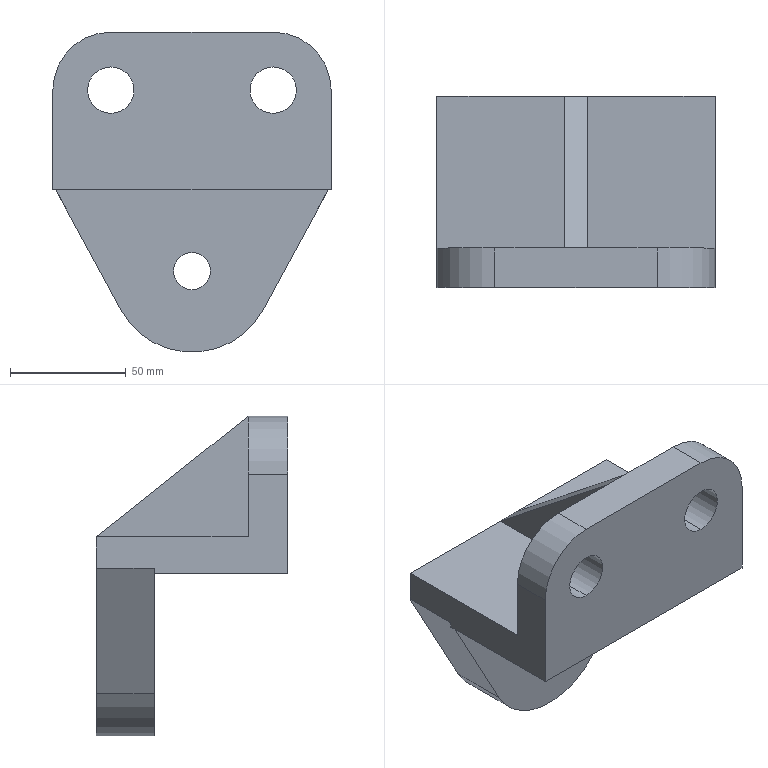Part | SolidWorks | features ICE 5, Extrusion 1 | 1 solid | 27 faces | box 120 x 82.471 x 138 mm | volume 396797 mm3 | plane 18 | cylinder 9 | commonest cylinder face diameters 20 x4 16 x2 50 x2 70 x1
STEP:
#1=CARTESIAN_POINT('',(-60.,57.471,-111.));
#2=VERTEX_POINT('',#1);
#3=CARTESIAN_POINT('',(-60.,57.471,-95.));
#4=VERTEX_POINT('',#3);
#5=CARTESIAN_POINT('',(-60.,57.471,-103.));
#6=DIRECTION('',(0.,1.,0.));
#7=DIRECTION('',(0.,0.,1.));
#8=AXIS2_PLACEMENT_3D('',#5,#6,#7);
#9=CIRCLE('',#8,8.);
#10=EDGE_CURVE('',#2,#4,#9,.T.);
#11=ORIENTED_EDGE('',*,*,#10,.F.);
#12=CARTESIAN_POINT('',(-60.,82.471,-111.));
#13=VERTEX_POINT('',#12);
#14=CARTESIAN_POINT('',(-60.,57.471,-111.));
#15=DIRECTION('',(0.,1.,0.));
#16=VECTOR('',#15,1000.);
#17=LINE('',#14,#16);
#18=EDGE_CURVE('',#2,#13,#17,.T.);
#19=ORIENTED_EDGE('',*,*,#18,.T.);
#20=CARTESIAN_POINT('',(-60.,82.471,-95.));
#21=VERTEX_POINT('',#20);
#22=CARTESIAN_POINT('',(-60.,82.471,-103.));
#23=DIRECTION('',(0.,1.,0.));
#24=DIRECTION('',(0.,0.,1.));
#25=AXIS2_PLACEMENT_3D('',#22,#23,#24);
#26=CIRCLE('',#25,8.);
#27=EDGE_CURVE('',#13,#21,#26,.T.);
#28=ORIENTED_EDGE('',*,*,#27,.T.);
#29=CARTESIAN_POINT('',(-60.,57.471,-95.));
#30=DIRECTION('',(0.,1.,0.));
#31=VECTOR('',#30,1000.);
#32=LINE('',#29,#31);
#33=EDGE_CURVE('',#4,#21,#32,.T.);
#34=ORIENTED_EDGE('',*,*,#33,.F.);
#35=EDGE_LOOP('',(#11,#19,#28,#34));
#36=FACE_OUTER_BOUND('',#35,.T.);
#37=CARTESIAN_POINT('',(-60.,57.471,-103.));
#38=DIRECTION('',(0.,1.,0.));
#39=DIRECTION('',(0.,0.,1.));
#40=AXIS2_PLACEMENT_3D('',#37,#38,#39);
#41=CYLINDRICAL_SURFACE('',#40,8.);
#42=ADVANCED_FACE('',(#36),#41,.F.);
#43=CARTESIAN_POINT('',(-25.,17.,-15.));
#44=VERTEX_POINT('',#43);
#45=CARTESIAN_POINT('',(-25.,17.,-35.));
#46=VERTEX_POINT('',#45);
#47=CARTESIAN_POINT('',(-25.,17.,-25.));
#48=DIRECTION('',(0.,-1.,0.));
#49=DIRECTION('',(0.,0.,-1.));
#50=AXIS2_PLACEMENT_3D('',#47,#48,#49);
#51=CIRCLE('',#50,10.);
#52=EDGE_CURVE('',#44,#46,#51,.T.);
#53=ORIENTED_EDGE('',*,*,#52,.F.);
#54=CARTESIAN_POINT('',(-25.,0.,-15.));
#55=VERTEX_POINT('',#54);
#56=CARTESIAN_POINT('',(-25.,55.,-15.));
#57=DIRECTION('',(0.,-1.,0.));
#58=VECTOR('',#57,1000.);
#59=LINE('',#56,#58);
#60=EDGE_CURVE('',#44,#55,#59,.T.);
#61=ORIENTED_EDGE('',*,*,#60,.T.);
#62=CARTESIAN_POINT('',(-25.,0.,-35.));
#63=VERTEX_POINT('',#62);
#64=CARTESIAN_POINT('',(-25.,0.,-25.));
#65=DIRECTION('',(0.,-1.,0.));
#66=DIRECTION('',(0.,0.,-1.));
#67=AXIS2_PLACEMENT_3D('',#64,#65,#66);
#68=CIRCLE('',#67,10.);
#69=EDGE_CURVE('',#55,#63,#68,.T.);
#70=ORIENTED_EDGE('',*,*,#69,.T.);
#71=CARTESIAN_POINT('',(-25.,55.,-35.));
#72=DIRECTION('',(0.,-1.,0.));
#73=VECTOR('',#72,1000.);
#74=LINE('',#71,#73);
#75=EDGE_CURVE('',#46,#63,#74,.T.);
#76=ORIENTED_EDGE('',*,*,#75,.F.);
#77=EDGE_LOOP('',(#53,#61,#70,#76));
#78=FACE_OUTER_BOUND('',#77,.T.);
#79=CARTESIAN_POINT('',(-25.,55.,-25.));
#80=DIRECTION('',(0.,-1.,0.));
#81=DIRECTION('',(0.,0.,-1.));
#82=AXIS2_PLACEMENT_3D('',#79,#80,#81);
#83=CYLINDRICAL_SURFACE('',#82,10.);
#84=ADVANCED_FACE('',(#78),#83,.F.);
#85=CARTESIAN_POINT('',(-95.,17.,-15.));
#86=VERTEX_POINT('',#85);
#87=CARTESIAN_POINT('',(-95.,17.,-35.));
#88=VERTEX_POINT('',#87);
#89=CARTESIAN_POINT('',(-95.,17.,-25.));
#90=DIRECTION('',(0.,-1.,0.));
#91=DIRECTION('',(0.,0.,-1.));
#92=AXIS2_PLACEMENT_3D('',#89,#90,#91);
#93=CIRCLE('',#92,10.);
#94=EDGE_CURVE('',#86,#88,#93,.T.);
#95=ORIENTED_EDGE('',*,*,#94,.F.);
#96=CARTESIAN_POINT('',(-95.,0.,-15.));
#97=VERTEX_POINT('',#96);
#98=CARTESIAN_POINT('',(-95.,55.,-15.));
#99=DIRECTION('',(0.,-1.,0.));
#100=VECTOR('',#99,1000.);
#101=LINE('',#98,#100);
#102=EDGE_CURVE('',#86,#97,#101,.T.);
#103=ORIENTED_EDGE('',*,*,#102,.T.);
#104=CARTESIAN_POINT('',(-95.,0.,-35.));
#105=VERTEX_POINT('',#104);
#106=CARTESIAN_POINT('',(-95.,0.,-25.));
#107=DIRECTION('',(0.,-1.,0.));
#108=DIRECTION('',(0.,0.,-1.));
#109=AXIS2_PLACEMENT_3D('',#106,#107,#108);
#110=CIRCLE('',#109,10.);
#111=EDGE_CURVE('',#97,#105,#110,.T.);
#112=ORIENTED_EDGE('',*,*,#111,.T.);
#113=CARTESIAN_POINT('',(-95.,55.,-35.));
#114=DIRECTION('',(0.,-1.,0.));
#115=VECTOR('',#114,1000.);
#116=LINE('',#113,#115);
#117=EDGE_CURVE('',#88,#105,#116,.T.);
#118=ORIENTED_EDGE('',*,*,#117,.F.);
#119=EDGE_LOOP('',(#95,#103,#112,#118));
#120=FACE_OUTER_BOUND('',#119,.T.);
#121=CARTESIAN_POINT('',(-95.,55.,-25.));
#122=DIRECTION('',(0.,-1.,0.));
#123=DIRECTION('',(0.,0.,-1.));
#124=AXIS2_PLACEMENT_3D('',#121,#122,#123);
#125=CYLINDRICAL_SURFACE('',#124,10.);
#126=ADVANCED_FACE('',(#120),#125,.F.);
#127=CARTESIAN_POINT('',(-60.,82.471,-103.));
#128=DIRECTION('',(0.,1.,0.));
#129=DIRECTION('',(0.,0.,1.));
#130=AXIS2_PLACEMENT_3D('',#127,#128,#129);
#131=CIRCLE('',#130,8.);
#132=EDGE_CURVE('',#21,#13,#131,.T.);
#133=ORIENTED_EDGE('',*,*,#132,.F.);
#134=ORIENTED_EDGE('',*,*,#27,.F.);
#135=EDGE_LOOP('',(#133,#134));
#136=FACE_BOUND('',#135,.T.);
#137=CARTESIAN_POINT('',(-29.216,82.471,-119.654));
#138=VERTEX_POINT('',#137);
#139=CARTESIAN_POINT('',(-90.784,82.471,-119.654));
#140=VERTEX_POINT('',#139);
#141=CARTESIAN_POINT('',(-60.,82.471,-103.));
#142=DIRECTION('',(0.,1.,0.));
#143=DIRECTION('',(0.,0.,1.));
#144=AXIS2_PLACEMENT_3D('',#141,#142,#143);
#145=CIRCLE('',#144,35.);
#146=EDGE_CURVE('',#138,#140,#145,.T.);
#147=ORIENTED_EDGE('',*,*,#146,.T.);
#148=CARTESIAN_POINT('',(-120.,82.471,-65.649));
#149=VERTEX_POINT('',#148);
#150=CARTESIAN_POINT('',(-120.306,82.471,-65.085));
#151=DIRECTION('',(0.4758,0.,-0.8795));
#152=VECTOR('',#151,1000.);
#153=LINE('',#150,#152);
#154=EDGE_CURVE('',#149,#140,#153,.T.);
#155=ORIENTED_EDGE('',*,*,#154,.F.);
#156=CARTESIAN_POINT('',(-120.,82.471,-52.));
#157=VERTEX_POINT('',#156);
#158=CARTESIAN_POINT('',(-120.,82.471,0.));
#159=DIRECTION('',(0.,0.,1.));
#160=VECTOR('',#159,1000.);
#161=LINE('',#158,#160);
#162=EDGE_CURVE('',#149,#157,#161,.T.);
#163=ORIENTED_EDGE('',*,*,#162,.T.);
#164=CARTESIAN_POINT('',(-65.,82.471,-52.));
#165=VERTEX_POINT('',#164);
#166=CARTESIAN_POINT('',(-120.,82.471,-52.));
#167=DIRECTION('',(1.,0.,0.));
#168=VECTOR('',#167,1000.);
#169=LINE('',#166,#168);
#170=EDGE_CURVE('',#157,#165,#169,.T.);
#171=ORIENTED_EDGE('',*,*,#170,.T.);
#172=CARTESIAN_POINT('',(-55.,82.471,-52.));
#173=VERTEX_POINT('',#172);
#174=CARTESIAN_POINT('',(-120.,82.471,-52.));
#175=DIRECTION('',(1.,0.,0.));
#176=VECTOR('',#175,1000.);
#177=LINE('',#174,#176);
#178=EDGE_CURVE('',#165,#173,#177,.T.);
#179=ORIENTED_EDGE('',*,*,#178,.T.);
#180=CARTESIAN_POINT('',(0.,82.471,-52.));
#181=VERTEX_POINT('',#180);
#182=CARTESIAN_POINT('',(-55.,82.471,-52.));
#183=DIRECTION('',(1.,0.,0.));
#184=VECTOR('',#183,1000.);
#185=LINE('',#182,#184);
#186=EDGE_CURVE('',#173,#181,#185,.T.);
#187=ORIENTED_EDGE('',*,*,#186,.T.);
#188=CARTESIAN_POINT('',(0.,82.471,-65.649));
#189=VERTEX_POINT('',#188);
#190=CARTESIAN_POINT('',(0.,82.471,0.));
#191=DIRECTION('',(0.,0.,1.));
#192=VECTOR('',#191,1000.);
#193=LINE('',#190,#192);
#194=EDGE_CURVE('',#189,#181,#193,.T.);
#195=ORIENTED_EDGE('',*,*,#194,.F.);
#196=CARTESIAN_POINT('',(27.475,82.471,-14.864));
#197=DIRECTION('',(-0.4758,0.,-0.8795));
#198=VECTOR('',#197,1000.);
#199=LINE('',#196,#198);
#200=EDGE_CURVE('',#189,#138,#199,.T.);
#201=ORIENTED_EDGE('',*,*,#200,.T.);
#202=EDGE_LOOP('',(#147,#155,#163,#171,#179,#187,#195,#201));
#203=FACE_OUTER_BOUND('',#202,.T.);
#204=CARTESIAN_POINT('',(-120.,82.471,0.));
#205=DIRECTION('',(0.,1.,0.));
#206=DIRECTION('',(0.,0.,1.));
#207=AXIS2_PLACEMENT_3D('',#204,#205,#206);
#208=PLANE('',#207);
#209=ADVANCED_FACE('',(#136,#203),#208,.T.);
#210=CARTESIAN_POINT('',(-60.,57.471,-103.));
#211=DIRECTION('',(0.,1.,0.));
#212=DIRECTION('',(0.,0.,1.));
#213=AXIS2_PLACEMENT_3D('',#210,#211,#212);
#214=CIRCLE('',#213,8.);
#215=EDGE_CURVE('',#4,#2,#214,.T.);
#216=ORIENTED_EDGE('',*,*,#215,.T.);
#217=ORIENTED_EDGE('',*,*,#10,.T.);
#218=EDGE_LOOP('',(#216,#217));
#219=FACE_BOUND('',#218,.T.);
#220=CARTESIAN_POINT('',(-118.728,57.471,-68.));
#221=VERTEX_POINT('',#220);
#222=CARTESIAN_POINT('',(-90.784,57.471,-119.654));
#223=VERTEX_POINT('',#222);
#224=CARTESIAN_POINT('',(-120.306,57.471,-65.085));
#225=DIRECTION('',(0.4758,0.,-0.8795));
#226=VECTOR('',#225,1000.);
#227=LINE('',#224,#226);
#228=EDGE_CURVE('',#221,#223,#227,.T.);
#229=ORIENTED_EDGE('',*,*,#228,.T.);
#230=CARTESIAN_POINT('',(-29.216,57.471,-119.654));
#231=VERTEX_POINT('',#230);
#232=CARTESIAN_POINT('',(-60.,57.471,-103.));
#233=DIRECTION('',(0.,1.,0.));
#234=DIRECTION('',(0.,0.,1.));
#235=AXIS2_PLACEMENT_3D('',#232,#233,#234);
#236=CIRCLE('',#235,35.);
#237=EDGE_CURVE('',#231,#223,#236,.T.);
#238=ORIENTED_EDGE('',*,*,#237,.F.);
#239=CARTESIAN_POINT('',(-1.272,57.471,-68.));
#240=VERTEX_POINT('',#239);
#241=CARTESIAN_POINT('',(-57.448,57.471,-171.84));
#242=DIRECTION('',(0.4758,0.,0.8795));
#243=VECTOR('',#242,1000.);
#244=LINE('',#241,#243);
#245=EDGE_CURVE('',#231,#240,#244,.T.);
#246=ORIENTED_EDGE('',*,*,#245,.T.);
#247=CARTESIAN_POINT('',(-120.,57.471,-68.));
#248=DIRECTION('',(1.,0.,0.));
#249=VECTOR('',#248,1000.);
#250=LINE('',#247,#249);
#251=EDGE_CURVE('',#221,#240,#250,.T.);
#252=ORIENTED_EDGE('',*,*,#251,.F.);
#253=EDGE_LOOP('',(#229,#238,#246,#252));
#254=FACE_OUTER_BOUND('',#253,.T.);
#255=CARTESIAN_POINT('',(-120.,57.471,-138.));
#256=DIRECTION('',(0.,-1.,0.));
#257=DIRECTION('',(0.,0.,-1.));
#258=AXIS2_PLACEMENT_3D('',#255,#256,#257);
#259=PLANE('',#258);
#260=ADVANCED_FACE('',(#219,#254),#259,.T.);
#261=CARTESIAN_POINT('',(0.,57.471,-65.649));
#262=VERTEX_POINT('',#261);
#263=CARTESIAN_POINT('',(0.,57.471,-68.));
#264=VERTEX_POINT('',#263);
#265=CARTESIAN_POINT('',(0.,57.471,0.));
#266=DIRECTION('',(0.,0.,-1.));
#267=VECTOR('',#266,1000.);
#268=LINE('',#265,#267);
#269=EDGE_CURVE('',#262,#264,#268,.T.);
#270=ORIENTED_EDGE('',*,*,#269,.F.);
#271=CARTESIAN_POINT('',(0.,57.471,-65.649));
#272=DIRECTION('',(0.,1.,0.));
#273=VECTOR('',#272,1000.);
#274=LINE('',#271,#273);
#275=EDGE_CURVE('',#262,#189,#274,.T.);
#276=ORIENTED_EDGE('',*,*,#275,.T.);
#277=ORIENTED_EDGE('',*,*,#194,.T.);
#278=CARTESIAN_POINT('',(0.,17.,-52.));
#279=VERTEX_POINT('',#278);
#280=CARTESIAN_POINT('',(0.,17.,-52.));
#281=DIRECTION('',(0.,1.,0.));
#282=VECTOR('',#281,1000.);
#283=LINE('',#280,#282);
#284=EDGE_CURVE('',#279,#181,#283,.T.);
#285=ORIENTED_EDGE('',*,*,#284,.F.);
#286=CARTESIAN_POINT('',(0.,17.,-25.));
#287=VERTEX_POINT('',#286);
#288=CARTESIAN_POINT('',(0.,17.,0.));
#289=DIRECTION('',(0.,0.,-1.));
#290=VECTOR('',#289,1000.);
#291=LINE('',#288,#290);
#292=EDGE_CURVE('',#287,#279,#291,.T.);
#293=ORIENTED_EDGE('',*,*,#292,.F.);
#294=CARTESIAN_POINT('',(0.,0.,-25.));
#295=VERTEX_POINT('',#294);
#296=CARTESIAN_POINT('',(0.,55.,-25.));
#297=DIRECTION('',(0.,-1.,0.));
#298=VECTOR('',#297,1000.);
#299=LINE('',#296,#298);
#300=EDGE_CURVE('',#287,#295,#299,.T.);
#301=ORIENTED_EDGE('',*,*,#300,.T.);
#302=CARTESIAN_POINT('',(0.,0.,-68.));
#303=VERTEX_POINT('',#302);
#304=CARTESIAN_POINT('',(0.,0.,0.));
#305=DIRECTION('',(0.,0.,-1.));
#306=VECTOR('',#305,1000.);
#307=LINE('',#304,#306);
#308=EDGE_CURVE('',#295,#303,#307,.T.);
#309=ORIENTED_EDGE('',*,*,#308,.T.);
#310=CARTESIAN_POINT('',(0.,0.,-68.));
#311=DIRECTION('',(0.,1.,0.));
#312=VECTOR('',#311,1000.);
#313=LINE('',#310,#312);
#314=EDGE_CURVE('',#303,#264,#313,.T.);
#315=ORIENTED_EDGE('',*,*,#314,.T.);
#316=EDGE_LOOP('',(#270,#276,#277,#285,#293,#301,#309,#315));
#317=FACE_OUTER_BOUND('',#316,.T.);
#318=CARTESIAN_POINT('',(0.,0.,0.));
#319=DIRECTION('',(1.,0.,0.));
#320=DIRECTION('',(0.,0.,-1.));
#321=AXIS2_PLACEMENT_3D('',#318,#319,#320);
#322=PLANE('',#321);
#323=ADVANCED_FACE('',(#317),#322,.T.);
#324=CARTESIAN_POINT('',(-120.,0.,-68.));
#325=VERTEX_POINT('',#324);
#326=CARTESIAN_POINT('',(-120.,57.471,-68.));
#327=VERTEX_POINT('',#326);
#328=CARTESIAN_POINT('',(-120.,0.,-68.));
#329=DIRECTION('',(0.,1.,0.));
#330=VECTOR('',#329,1000.);
#331=LINE('',#328,#330);
#332=EDGE_CURVE('',#325,#327,#331,.T.);
#333=ORIENTED_EDGE('',*,*,#332,.T.);
#334=CARTESIAN_POINT('',(-120.,57.471,-68.));
#335=DIRECTION('',(1.,0.,0.));
#336=VECTOR('',#335,1000.);
#337=LINE('',#334,#336);
#338=EDGE_CURVE('',#327,#221,#337,.T.);
#339=ORIENTED_EDGE('',*,*,#338,.T.);
#340=ORIENTED_EDGE('',*,*,#251,.T.);
#341=CARTESIAN_POINT('',(-120.,57.471,-68.));
#342=DIRECTION('',(1.,0.,0.));
#343=VECTOR('',#342,1000.);
#344=LINE('',#341,#343);
#345=EDGE_CURVE('',#240,#264,#344,.T.);
#346=ORIENTED_EDGE('',*,*,#345,.T.);
#347=ORIENTED_EDGE('',*,*,#314,.F.);
#348=CARTESIAN_POINT('',(-120.,0.,-68.));
#349=DIRECTION('',(1.,0.,0.));
#350=VECTOR('',#349,1000.);
#351=LINE('',#348,#350);
#352=EDGE_CURVE('',#325,#303,#351,.T.);
#353=ORIENTED_EDGE('',*,*,#352,.F.);
#354=EDGE_LOOP('',(#333,#339,#340,#346,#347,#353));
#355=FACE_OUTER_BOUND('',#354,.T.);
#356=CARTESIAN_POINT('',(-120.,0.,-68.));
#357=DIRECTION('',(0.,0.,-1.));
#358=DIRECTION('',(-1.,0.,0.));
#359=AXIS2_PLACEMENT_3D('',#356,#357,#358);
#360=PLANE('',#359);
#361=ADVANCED_FACE('',(#355),#360,.T.);
#362=CARTESIAN_POINT('',(-25.,0.,-25.));
#363=DIRECTION('',(0.,-1.,0.));
#364=DIRECTION('',(0.,0.,-1.));
#365=AXIS2_PLACEMENT_3D('',#362,#363,#364);
#366=CIRCLE('',#365,10.);
#367=EDGE_CURVE('',#63,#55,#366,.T.);
#368=ORIENTED_EDGE('',*,*,#367,.F.);
#369=ORIENTED_EDGE('',*,*,#69,.F.);
#370=EDGE_LOOP('',(#368,#369));
#371=FACE_BOUND('',#370,.T.);
#372=CARTESIAN_POINT('',(-95.,0.,-25.));
#373=DIRECTION('',(0.,-1.,0.));
#374=DIRECTION('',(0.,0.,-1.));
#375=AXIS2_PLACEMENT_3D('',#372,#373,#374);
#376=CIRCLE('',#375,10.);
#377=EDGE_CURVE('',#105,#97,#376,.T.);
#378=ORIENTED_EDGE('',*,*,#377,.F.);
#379=ORIENTED_EDGE('',*,*,#111,.F.);
#380=EDGE_LOOP('',(#378,#379));
#381=FACE_BOUND('',#380,.T.);
#382=ORIENTED_EDGE('',*,*,#308,.F.);
#383=CARTESIAN_POINT('',(-25.,0.,0.));
#384=VERTEX_POINT('',#383);
#385=CARTESIAN_POINT('',(-25.,0.,-25.));
#386=DIRECTION('',(0.,-1.,0.));
#387=DIRECTION('',(0.,0.,-1.));
#388=AXIS2_PLACEMENT_3D('',#385,#386,#387);
#389=CIRCLE('',#388,25.);
#390=EDGE_CURVE('',#295,#384,#389,.T.);
#391=ORIENTED_EDGE('',*,*,#390,.T.);
#392=CARTESIAN_POINT('',(-95.,0.,0.));
#393=VERTEX_POINT('',#392);
#394=CARTESIAN_POINT('',(-120.,0.,0.));
#395=DIRECTION('',(1.,0.,0.));
#396=VECTOR('',#395,1000.);
#397=LINE('',#394,#396);
#398=EDGE_CURVE('',#393,#384,#397,.T.);
#399=ORIENTED_EDGE('',*,*,#398,.F.);
#400=CARTESIAN_POINT('',(-120.,0.,-25.));
#401=VERTEX_POINT('',#400);
#402=CARTESIAN_POINT('',(-95.,0.,-25.));
#403=DIRECTION('',(0.,-1.,0.));
#404=DIRECTION('',(0.,0.,-1.));
#405=AXIS2_PLACEMENT_3D('',#402,#403,#404);
#406=CIRCLE('',#405,25.);
#407=EDGE_CURVE('',#393,#401,#406,.T.);
#408=ORIENTED_EDGE('',*,*,#407,.T.);
#409=CARTESIAN_POINT('',(-120.,0.,0.));
#410=DIRECTION('',(0.,0.,-1.));
#411=VECTOR('',#410,1000.);
#412=LINE('',#409,#411);
#413=EDGE_CURVE('',#401,#325,#412,.T.);
#414=ORIENTED_EDGE('',*,*,#413,.T.);
#415=ORIENTED_EDGE('',*,*,#352,.T.);
#416=EDGE_LOOP('',(#382,#391,#399,#408,#414,#415));
#417=FACE_OUTER_BOUND('',#416,.T.);
#418=CARTESIAN_POINT('',(-120.,0.,0.));
#419=DIRECTION('',(0.,-1.,0.));
#420=DIRECTION('',(0.,0.,-1.));
#421=AXIS2_PLACEMENT_3D('',#418,#419,#420);
#422=PLANE('',#421);
#423=ADVANCED_FACE('',(#371,#381,#417),#422,.T.);
#424=CARTESIAN_POINT('',(-25.,17.,-25.));
#425=DIRECTION('',(0.,-1.,0.));
#426=DIRECTION('',(0.,0.,-1.));
#427=AXIS2_PLACEMENT_3D('',#424,#425,#426);
#428=CIRCLE('',#427,10.);
#429=EDGE_CURVE('',#46,#44,#428,.T.);
#430=ORIENTED_EDGE('',*,*,#429,.T.);
#431=ORIENTED_EDGE('',*,*,#52,.T.);
#432=EDGE_LOOP('',(#430,#431));
#433=FACE_BOUND('',#432,.T.);
#434=CARTESIAN_POINT('',(-25.,17.,0.));
#435=VERTEX_POINT('',#434);
#436=CARTESIAN_POINT('',(-25.,17.,-25.));
#437=DIRECTION('',(0.,-1.,0.));
#438=DIRECTION('',(0.,0.,-1.));
#439=AXIS2_PLACEMENT_3D('',#436,#437,#438);
#440=CIRCLE('',#439,25.);
#441=EDGE_CURVE('',#287,#435,#440,.T.);
#442=ORIENTED_EDGE('',*,*,#441,.F.);
#443=ORIENTED_EDGE('',*,*,#292,.T.);
#444=CARTESIAN_POINT('',(-55.,17.,-52.));
#445=VERTEX_POINT('',#444);
#446=CARTESIAN_POINT('',(-55.,17.,-52.));
#447=DIRECTION('',(1.,0.,0.));
#448=VECTOR('',#447,1000.);
#449=LINE('',#446,#448);
#450=EDGE_CURVE('',#445,#279,#449,.T.);
#451=ORIENTED_EDGE('',*,*,#450,.F.);
#452=CARTESIAN_POINT('',(-55.,17.,0.));
#453=VERTEX_POINT('',#452);
#454=CARTESIAN_POINT('',(-55.,17.,0.));
#455=DIRECTION('',(0.,0.,-1.));
#456=VECTOR('',#455,1000.);
#457=LINE('',#454,#456);
#458=EDGE_CURVE('',#453,#445,#457,.T.);
#459=ORIENTED_EDGE('',*,*,#458,.F.);
#460=CARTESIAN_POINT('',(-55.,17.,0.));
#461=DIRECTION('',(1.,0.,0.));
#462=VECTOR('',#461,1000.);
#463=LINE('',#460,#462);
#464=EDGE_CURVE('',#453,#435,#463,.T.);
#465=ORIENTED_EDGE('',*,*,#464,.T.);
#466=EDGE_LOOP('',(#442,#443,#451,#459,#465));
#467=FACE_OUTER_BOUND('',#466,.T.);
#468=CARTESIAN_POINT('',(-55.,17.,0.));
#469=DIRECTION('',(0.,-1.,0.));
#470=DIRECTION('',(0.,0.,-1.));
#471=AXIS2_PLACEMENT_3D('',#468,#469,#470);
#472=PLANE('',#471);
#473=ADVANCED_FACE('',(#433,#467),#472,.F.);
#474=CARTESIAN_POINT('',(-25.,55.,0.));
#475=DIRECTION('',(0.,-1.,0.));
#476=VECTOR('',#475,1000.);
#477=LINE('',#474,#476);
#478=EDGE_CURVE('',#435,#384,#477,.T.);
#479=ORIENTED_EDGE('',*,*,#478,.F.);
#480=ORIENTED_EDGE('',*,*,#464,.F.);
#481=CARTESIAN_POINT('',(-65.,17.,0.));
#482=VERTEX_POINT('',#481);
#483=CARTESIAN_POINT('',(-120.,17.,0.));
#484=DIRECTION('',(1.,0.,0.));
#485=VECTOR('',#484,1000.);
#486=LINE('',#483,#485);
#487=EDGE_CURVE('',#482,#453,#486,.T.);
#488=ORIENTED_EDGE('',*,*,#487,.F.);
#489=CARTESIAN_POINT('',(-95.,17.,0.));
#490=VERTEX_POINT('',#489);
#491=CARTESIAN_POINT('',(-120.,17.,0.));
#492=DIRECTION('',(1.,0.,0.));
#493=VECTOR('',#492,1000.);
#494=LINE('',#491,#493);
#495=EDGE_CURVE('',#490,#482,#494,.T.);
#496=ORIENTED_EDGE('',*,*,#495,.F.);
#497=CARTESIAN_POINT('',(-95.,55.,0.));
#498=DIRECTION('',(0.,-1.,0.));
#499=VECTOR('',#498,1000.);
#500=LINE('',#497,#499);
#501=EDGE_CURVE('',#490,#393,#500,.T.);
#502=ORIENTED_EDGE('',*,*,#501,.T.);
#503=ORIENTED_EDGE('',*,*,#398,.T.);
#504=EDGE_LOOP('',(#479,#480,#488,#496,#502,#503));
#505=FACE_OUTER_BOUND('',#504,.T.);
#506=CARTESIAN_POINT('',(-120.,0.,0.));
#507=DIRECTION('',(0.,0.,1.));
#508=DIRECTION('',(0.,-1.,0.));
#509=AXIS2_PLACEMENT_3D('',#506,#507,#508);
#510=PLANE('',#509);
#511=ADVANCED_FACE('',(#505),#510,.T.);
#512=ORIENTED_EDGE('',*,*,#162,.F.);
#513=CARTESIAN_POINT('',(-120.,57.471,-65.649));
#514=VERTEX_POINT('',#513);
#515=CARTESIAN_POINT('',(-120.,57.471,-65.649));
#516=DIRECTION('',(0.,1.,0.));
#517=VECTOR('',#516,1000.);
#518=LINE('',#515,#517);
#519=EDGE_CURVE('',#514,#149,#518,.T.);
#520=ORIENTED_EDGE('',*,*,#519,.F.);
#521=CARTESIAN_POINT('',(-120.,57.471,0.));
#522=DIRECTION('',(0.,0.,1.));
#523=VECTOR('',#522,1000.);
#524=LINE('',#521,#523);
#525=EDGE_CURVE('',#327,#514,#524,.T.);
#526=ORIENTED_EDGE('',*,*,#525,.F.);
#527=ORIENTED_EDGE('',*,*,#332,.F.);
#528=ORIENTED_EDGE('',*,*,#413,.F.);
#529=CARTESIAN_POINT('',(-120.,17.,-25.));
#530=VERTEX_POINT('',#529);
#531=CARTESIAN_POINT('',(-120.,55.,-25.));
#532=DIRECTION('',(0.,-1.,0.));
#533=VECTOR('',#532,1000.);
#534=LINE('',#531,#533);
#535=EDGE_CURVE('',#530,#401,#534,.T.);
#536=ORIENTED_EDGE('',*,*,#535,.F.);
#537=CARTESIAN_POINT('',(-120.,17.,-52.));
#538=VERTEX_POINT('',#537);
#539=CARTESIAN_POINT('',(-120.,17.,0.));
#540=DIRECTION('',(0.,0.,1.));
#541=VECTOR('',#540,1000.);
#542=LINE('',#539,#541);
#543=EDGE_CURVE('',#538,#530,#542,.T.);
#544=ORIENTED_EDGE('',*,*,#543,.F.);
#545=CARTESIAN_POINT('',(-120.,17.,-52.));
#546=DIRECTION('',(0.,-1.,0.));
#547=VECTOR('',#546,1000.);
#548=LINE('',#545,#547);
#549=EDGE_CURVE('',#157,#538,#548,.T.);
#550=ORIENTED_EDGE('',*,*,#549,.F.);
#551=EDGE_LOOP('',(#512,#520,#526,#527,#528,#536,#544,#550));
#552=FACE_OUTER_BOUND('',#551,.T.);
#553=CARTESIAN_POINT('',(-120.,0.,0.));
#554=DIRECTION('',(1.,0.,0.));
#555=DIRECTION('',(0.,0.,-1.));
#556=AXIS2_PLACEMENT_3D('',#553,#554,#555);
#557=PLANE('',#556);
#558=ADVANCED_FACE('',(#552),#557,.F.);
#559=CARTESIAN_POINT('',(-95.,17.,-25.));
#560=DIRECTION('',(0.,-1.,0.));
#561=DIRECTION('',(0.,0.,-1.));
#562=AXIS2_PLACEMENT_3D('',#559,#560,#561);
#563=CIRCLE('',#562,10.);
#564=EDGE_CURVE('',#88,#86,#563,.T.);
#565=ORIENTED_EDGE('',*,*,#564,.T.);
#566=ORIENTED_EDGE('',*,*,#94,.T.);
#567=EDGE_LOOP('',(#565,#566));
#568=FACE_BOUND('',#567,.T.);
#569=CARTESIAN_POINT('',(-95.,17.,-25.));
#570=DIRECTION('',(0.,-1.,0.));
#571=DIRECTION('',(0.,0.,-1.));
#572=AXIS2_PLACEMENT_3D('',#569,#570,#571);
#573=CIRCLE('',#572,25.);
#574=EDGE_CURVE('',#490,#530,#573,.T.);
#575=ORIENTED_EDGE('',*,*,#574,.F.);
#576=ORIENTED_EDGE('',*,*,#495,.T.);
#577=CARTESIAN_POINT('',(-65.,17.,-52.));
#578=VERTEX_POINT('',#577);
#579=CARTESIAN_POINT('',(-65.,17.,0.));
#580=DIRECTION('',(0.,0.,1.));
#581=VECTOR('',#580,1000.);
#582=LINE('',#579,#581);
#583=EDGE_CURVE('',#578,#482,#582,.T.);
#584=ORIENTED_EDGE('',*,*,#583,.F.);
#585=CARTESIAN_POINT('',(-65.,17.,-52.));
#586=DIRECTION('',(-1.,0.,0.));
#587=VECTOR('',#586,1000.);
#588=LINE('',#585,#587);
#589=EDGE_CURVE('',#578,#538,#588,.T.);
#590=ORIENTED_EDGE('',*,*,#589,.T.);
#591=ORIENTED_EDGE('',*,*,#543,.T.);
#592=EDGE_LOOP('',(#575,#576,#584,#590,#591));
#593=FACE_OUTER_BOUND('',#592,.T.);
#594=CARTESIAN_POINT('',(-65.,17.,0.));
#595=DIRECTION('',(0.,-1.,0.));
#596=DIRECTION('',(0.,0.,-1.));
#597=AXIS2_PLACEMENT_3D('',#594,#595,#596);
#598=PLANE('',#597);
#599=ADVANCED_FACE('',(#568,#593),#598,.F.);
#600=ORIENTED_EDGE('',*,*,#178,.F.);
#601=CARTESIAN_POINT('',(-65.,82.471,-52.));
#602=DIRECTION('',(0.,0.7831,-0.6219));
#603=VECTOR('',#602,1000.);
#604=LINE('',#601,#603);
#605=EDGE_CURVE('',#482,#165,#604,.T.);
#606=ORIENTED_EDGE('',*,*,#605,.F.);
#607=ORIENTED_EDGE('',*,*,#487,.T.);
#608=CARTESIAN_POINT('',(-55.,82.471,-52.));
#609=DIRECTION('',(0.,-0.7831,0.6219));
#610=VECTOR('',#609,1000.);
#611=LINE('',#608,#610);
#612=EDGE_CURVE('',#173,#453,#611,.T.);
#613=ORIENTED_EDGE('',*,*,#612,.F.);
#614=EDGE_LOOP('',(#600,#606,#607,#613));
#615=FACE_OUTER_BOUND('',#614,.T.);
#616=CARTESIAN_POINT('',(-120.,6.576,8.279));
#617=DIRECTION('',(0.,0.6219,0.7831));
#618=DIRECTION('',(0.,-0.7831,0.6219));
#619=AXIS2_PLACEMENT_3D('',#616,#617,#618);
#620=PLANE('',#619);
#621=ADVANCED_FACE('',(#615),#620,.T.);
#622=ORIENTED_EDGE('',*,*,#284,.T.);
#623=ORIENTED_EDGE('',*,*,#186,.F.);
#624=CARTESIAN_POINT('',(-55.,17.,-52.));
#625=DIRECTION('',(0.,1.,0.));
#626=VECTOR('',#625,1000.);
#627=LINE('',#624,#626);
#628=EDGE_CURVE('',#445,#173,#627,.T.);
#629=ORIENTED_EDGE('',*,*,#628,.F.);
#630=ORIENTED_EDGE('',*,*,#450,.T.);
#631=EDGE_LOOP('',(#622,#623,#629,#630));
#632=FACE_OUTER_BOUND('',#631,.T.);
#633=CARTESIAN_POINT('',(-55.,17.,-52.));
#634=DIRECTION('',(0.,0.,-1.));
#635=DIRECTION('',(-1.,0.,0.));
#636=AXIS2_PLACEMENT_3D('',#633,#634,#635);
#637=PLANE('',#636);
#638=ADVANCED_FACE('',(#632),#637,.F.);
#639=ORIENTED_EDGE('',*,*,#628,.T.);
#640=ORIENTED_EDGE('',*,*,#612,.T.);
#641=ORIENTED_EDGE('',*,*,#458,.T.);
#642=EDGE_LOOP('',(#639,#640,#641));
#643=FACE_OUTER_BOUND('',#642,.T.);
#644=CARTESIAN_POINT('',(-55.,0.,0.));
#645=DIRECTION('',(-1.,0.,0.));
#646=DIRECTION('',(0.,0.,1.));
#647=AXIS2_PLACEMENT_3D('',#644,#645,#646);
#648=PLANE('',#647);
#649=ADVANCED_FACE('',(#643),#648,.F.);
#650=ORIENTED_EDGE('',*,*,#549,.T.);
#651=ORIENTED_EDGE('',*,*,#589,.F.);
#652=CARTESIAN_POINT('',(-65.,17.,-52.));
#653=DIRECTION('',(0.,-1.,0.));
#654=VECTOR('',#653,1000.);
#655=LINE('',#652,#654);
#656=EDGE_CURVE('',#165,#578,#655,.T.);
#657=ORIENTED_EDGE('',*,*,#656,.F.);
#658=ORIENTED_EDGE('',*,*,#170,.F.);
#659=EDGE_LOOP('',(#650,#651,#657,#658));
#660=FACE_OUTER_BOUND('',#659,.T.);
#661=CARTESIAN_POINT('',(-65.,17.,-52.));
#662=DIRECTION('',(0.,0.,-1.));
#663=DIRECTION('',(-1.,0.,0.));
#664=AXIS2_PLACEMENT_3D('',#661,#662,#663);
#665=PLANE('',#664);
#666=ADVANCED_FACE('',(#660),#665,.F.);
#667=ORIENTED_EDGE('',*,*,#656,.T.);
#668=ORIENTED_EDGE('',*,*,#583,.T.);
#669=ORIENTED_EDGE('',*,*,#605,.T.);
#670=EDGE_LOOP('',(#667,#668,#669));
#671=FACE_OUTER_BOUND('',#670,.T.);
#672=CARTESIAN_POINT('',(-65.,0.,0.));
#673=DIRECTION('',(-1.,0.,0.));
#674=DIRECTION('',(0.,0.,1.));
#675=AXIS2_PLACEMENT_3D('',#672,#673,#674);
#676=PLANE('',#675);
#677=ADVANCED_FACE('',(#671),#676,.T.);
#678=ORIENTED_EDGE('',*,*,#102,.F.);
#679=ORIENTED_EDGE('',*,*,#564,.F.);
#680=ORIENTED_EDGE('',*,*,#117,.T.);
#681=ORIENTED_EDGE('',*,*,#377,.T.);
#682=EDGE_LOOP('',(#678,#679,#680,#681));
#683=FACE_OUTER_BOUND('',#682,.T.);
#684=CARTESIAN_POINT('',(-95.,55.,-25.));
#685=DIRECTION('',(0.,-1.,0.));
#686=DIRECTION('',(0.,0.,-1.));
#687=AXIS2_PLACEMENT_3D('',#684,#685,#686);
#688=CYLINDRICAL_SURFACE('',#687,10.);
#689=ADVANCED_FACE('',(#683),#688,.F.);
#690=ORIENTED_EDGE('',*,*,#60,.F.);
#691=ORIENTED_EDGE('',*,*,#429,.F.);
#692=ORIENTED_EDGE('',*,*,#75,.T.);
#693=ORIENTED_EDGE('',*,*,#367,.T.);
#694=EDGE_LOOP('',(#690,#691,#692,#693));
#695=FACE_OUTER_BOUND('',#694,.T.);
#696=CARTESIAN_POINT('',(-25.,55.,-25.));
#697=DIRECTION('',(0.,-1.,0.));
#698=DIRECTION('',(0.,0.,-1.));
#699=AXIS2_PLACEMENT_3D('',#696,#697,#698);
#700=CYLINDRICAL_SURFACE('',#699,10.);
#701=ADVANCED_FACE('',(#695),#700,.F.);
#702=ORIENTED_EDGE('',*,*,#574,.T.);
#703=ORIENTED_EDGE('',*,*,#535,.T.);
#704=ORIENTED_EDGE('',*,*,#407,.F.);
#705=ORIENTED_EDGE('',*,*,#501,.F.);
#706=EDGE_LOOP('',(#702,#703,#704,#705));
#707=FACE_OUTER_BOUND('',#706,.T.);
#708=CARTESIAN_POINT('',(-95.,55.,-25.));
#709=DIRECTION('',(0.,-1.,0.));
#710=DIRECTION('',(0.,0.,-1.));
#711=AXIS2_PLACEMENT_3D('',#708,#709,#710);
#712=CYLINDRICAL_SURFACE('',#711,25.);
#713=ADVANCED_FACE('',(#707),#712,.T.);
#714=ORIENTED_EDGE('',*,*,#441,.T.);
#715=ORIENTED_EDGE('',*,*,#478,.T.);
#716=ORIENTED_EDGE('',*,*,#390,.F.);
#717=ORIENTED_EDGE('',*,*,#300,.F.);
#718=EDGE_LOOP('',(#714,#715,#716,#717));
#719=FACE_OUTER_BOUND('',#718,.T.);
#720=CARTESIAN_POINT('',(-25.,55.,-25.));
#721=DIRECTION('',(0.,-1.,0.));
#722=DIRECTION('',(0.,0.,-1.));
#723=AXIS2_PLACEMENT_3D('',#720,#721,#722);
#724=CYLINDRICAL_SURFACE('',#723,25.);
#725=ADVANCED_FACE('',(#719),#724,.T.);
#726=ORIENTED_EDGE('',*,*,#18,.F.);
#727=ORIENTED_EDGE('',*,*,#215,.F.);
#728=ORIENTED_EDGE('',*,*,#33,.T.);
#729=ORIENTED_EDGE('',*,*,#132,.T.);
#730=EDGE_LOOP('',(#726,#727,#728,#729));
#731=FACE_OUTER_BOUND('',#730,.T.);
#732=CARTESIAN_POINT('',(-60.,57.471,-103.));
#733=DIRECTION('',(0.,1.,0.));
#734=DIRECTION('',(0.,0.,1.));
#735=AXIS2_PLACEMENT_3D('',#732,#733,#734);
#736=CYLINDRICAL_SURFACE('',#735,8.);
#737=ADVANCED_FACE('',(#731),#736,.F.);
#738=ORIENTED_EDGE('',*,*,#146,.F.);
#739=CARTESIAN_POINT('',(-29.216,57.471,-119.654));
#740=DIRECTION('',(0.,1.,0.));
#741=VECTOR('',#740,1000.);
#742=LINE('',#739,#741);
#743=EDGE_CURVE('',#231,#138,#742,.T.);
#744=ORIENTED_EDGE('',*,*,#743,.F.);
#745=ORIENTED_EDGE('',*,*,#237,.T.);
#746=CARTESIAN_POINT('',(-90.784,57.471,-119.654));
#747=DIRECTION('',(0.,1.,0.));
#748=VECTOR('',#747,1000.);
#749=LINE('',#746,#748);
#750=EDGE_CURVE('',#223,#140,#749,.T.);
#751=ORIENTED_EDGE('',*,*,#750,.T.);
#752=EDGE_LOOP('',(#738,#744,#745,#751));
#753=FACE_OUTER_BOUND('',#752,.T.);
#754=CARTESIAN_POINT('',(-60.,57.471,-103.));
#755=DIRECTION('',(0.,1.,0.));
#756=DIRECTION('',(0.,0.,1.));
#757=AXIS2_PLACEMENT_3D('',#754,#755,#756);
#758=CYLINDRICAL_SURFACE('',#757,35.);
#759=ADVANCED_FACE('',(#753),#758,.T.);
#760=ORIENTED_EDGE('',*,*,#200,.F.);
#761=ORIENTED_EDGE('',*,*,#275,.F.);
#762=CARTESIAN_POINT('',(27.475,57.471,-14.864));
#763=DIRECTION('',(-0.4758,0.,-0.8795));
#764=VECTOR('',#763,1000.);
#765=LINE('',#762,#764);
#766=EDGE_CURVE('',#262,#240,#765,.T.);
#767=ORIENTED_EDGE('',*,*,#766,.T.);
#768=ORIENTED_EDGE('',*,*,#245,.F.);
#769=ORIENTED_EDGE('',*,*,#743,.T.);
#770=EDGE_LOOP('',(#760,#761,#767,#768,#769));
#771=FACE_OUTER_BOUND('',#770,.T.);
#772=CARTESIAN_POINT('',(27.475,57.471,-14.864));
#773=DIRECTION('',(0.8795,0.,-0.4758));
#774=DIRECTION('',(-0.4758,0.,-0.8795));
#775=AXIS2_PLACEMENT_3D('',#772,#773,#774);
#776=PLANE('',#775);
#777=ADVANCED_FACE('',(#771),#776,.T.);
#778=ORIENTED_EDGE('',*,*,#766,.F.);
#779=ORIENTED_EDGE('',*,*,#269,.T.);
#780=ORIENTED_EDGE('',*,*,#345,.F.);
#781=EDGE_LOOP('',(#778,#779,#780));
#782=FACE_OUTER_BOUND('',#781,.T.);
#783=CARTESIAN_POINT('',(0.,57.471,0.));
#784=DIRECTION('',(0.,1.,0.));
#785=DIRECTION('',(0.,0.,1.));
#786=AXIS2_PLACEMENT_3D('',#783,#784,#785);
#787=PLANE('',#786);
#788=ADVANCED_FACE('',(#782),#787,.T.);
#789=ORIENTED_EDGE('',*,*,#154,.T.);
#790=ORIENTED_EDGE('',*,*,#750,.F.);
#791=ORIENTED_EDGE('',*,*,#228,.F.);
#792=CARTESIAN_POINT('',(-120.306,57.471,-65.085));
#793=DIRECTION('',(0.4758,0.,-0.8795));
#794=VECTOR('',#793,1000.);
#795=LINE('',#792,#794);
#796=EDGE_CURVE('',#514,#221,#795,.T.);
#797=ORIENTED_EDGE('',*,*,#796,.F.);
#798=ORIENTED_EDGE('',*,*,#519,.T.);
#799=EDGE_LOOP('',(#789,#790,#791,#797,#798));
#800=FACE_OUTER_BOUND('',#799,.T.);
#801=CARTESIAN_POINT('',(-120.306,57.471,-65.085));
#802=DIRECTION('',(0.8795,0.,0.4758));
#803=DIRECTION('',(0.4758,0.,-0.8795));
#804=AXIS2_PLACEMENT_3D('',#801,#802,#803);
#805=PLANE('',#804);
#806=ADVANCED_FACE('',(#800),#805,.F.);
#807=ORIENTED_EDGE('',*,*,#525,.T.);
#808=ORIENTED_EDGE('',*,*,#796,.T.);
#809=ORIENTED_EDGE('',*,*,#338,.F.);
#810=EDGE_LOOP('',(#807,#808,#809));
#811=FACE_OUTER_BOUND('',#810,.T.);
#812=CARTESIAN_POINT('',(0.,57.471,0.));
#813=DIRECTION('',(0.,1.,0.));
#814=DIRECTION('',(0.,0.,1.));
#815=AXIS2_PLACEMENT_3D('',#812,#813,#814);
#816=PLANE('',#815);
#817=ADVANCED_FACE('',(#811),#816,.T.);
#818=CLOSED_SHELL('',(#42,#84,#126,#209,#260,#323,#361,#423,#473,#511,#558,#599,#621,#638,#649,#666,#677,#689,#701,#713,#725,#737,#759,#777,#788,#806,#817));
#819=MANIFOLD_SOLID_BREP('',#818);
#820=CARTESIAN_POINT('',(0.,0.,0.));
#821=DIRECTION('',(0.,0.,1.));
#822=DIRECTION('',(1.,0.,0.));
#823=AXIS2_PLACEMENT_3D('',#820,#821,#822);
#824=(LENGTH_UNIT()NAMED_UNIT(*)SI_UNIT(.MILLI.,.METRE.));
#825=UNCERTAINTY_MEASURE_WITH_UNIT(LENGTH_MEASURE(0.00001),#824,'','');
#826=(NAMED_UNIT(*)PLANE_ANGLE_UNIT()SI_UNIT($,.RADIAN.));
#827=(NAMED_UNIT(*)SI_UNIT($,.STERADIAN.)SOLID_ANGLE_UNIT());
#828=(GEOMETRIC_REPRESENTATION_CONTEXT(3)GLOBAL_UNCERTAINTY_ASSIGNED_CONTEXT((#825))GLOBAL_UNIT_ASSIGNED_CONTEXT((#824,#826,#827))REPRESENTATION_CONTEXT('',''));
#829=ADVANCED_BREP_SHAPE_REPRESENTATION('',(#819,#823),#828);